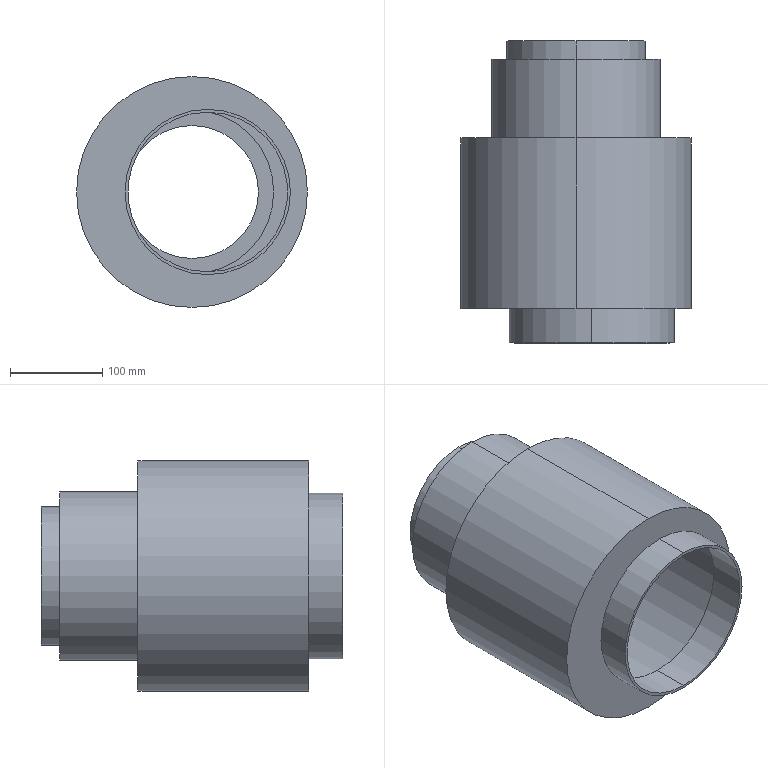Part | SolidWorks | features ICE 1, Revolution 1, Shell 1 | 1 solid | 24 faces | box 250 x 327 x 250 mm | volume 825128 mm3 | cylinder 16 | plane 8 | commonest cylinder face diameters 144 x2 150 x2 173 x2 177 x2 179 x2 183 x2
STEP:
#1=CARTESIAN_POINT('',(17.,-37.,86.5));
#2=VERTEX_POINT('',#1);
#3=CARTESIAN_POINT('',(17.,-37.,-86.5));
#4=VERTEX_POINT('',#3);
#5=CARTESIAN_POINT('',(17.,-37.,0.));
#6=DIRECTION('',(0.,-1.,0.));
#7=DIRECTION('',(0.,0.,-1.));
#8=AXIS2_PLACEMENT_3D('',#5,#6,#7);
#9=CIRCLE('',#8,86.5);
#10=EDGE_CURVE('',#2,#4,#9,.T.);
#11=ORIENTED_EDGE('',*,*,#10,.T.);
#12=CARTESIAN_POINT('',(17.,3.,-86.5));
#13=VERTEX_POINT('',#12);
#14=CARTESIAN_POINT('',(17.,-37.,-86.5));
#15=DIRECTION('',(0.,1.,0.));
#16=VECTOR('',#15,1000.);
#17=LINE('',#14,#16);
#18=EDGE_CURVE('',#4,#13,#17,.T.);
#19=ORIENTED_EDGE('',*,*,#18,.T.);
#20=CARTESIAN_POINT('',(17.,3.,86.5));
#21=VERTEX_POINT('',#20);
#22=CARTESIAN_POINT('',(17.,3.,0.));
#23=DIRECTION('',(0.,-1.,0.));
#24=DIRECTION('',(0.,0.,1.));
#25=AXIS2_PLACEMENT_3D('',#22,#23,#24);
#26=CIRCLE('',#25,86.5);
#27=EDGE_CURVE('',#21,#13,#26,.T.);
#28=ORIENTED_EDGE('',*,*,#27,.F.);
#29=CARTESIAN_POINT('',(17.,-37.,86.5));
#30=DIRECTION('',(0.,1.,0.));
#31=VECTOR('',#30,1000.);
#32=LINE('',#29,#31);
#33=EDGE_CURVE('',#2,#21,#32,.T.);
#34=ORIENTED_EDGE('',*,*,#33,.F.);
#35=EDGE_LOOP('',(#11,#19,#28,#34));
#36=FACE_OUTER_BOUND('',#35,.T.);
#37=CARTESIAN_POINT('',(17.,-37.,0.));
#38=DIRECTION('',(0.,1.,0.));
#39=DIRECTION('',(0.,0.,1.));
#40=AXIS2_PLACEMENT_3D('',#37,#38,#39);
#41=CYLINDRICAL_SURFACE('',#40,86.5);
#42=ADVANCED_FACE('',(#36),#41,.F.);
#43=CARTESIAN_POINT('',(0.,267.,-72.));
#44=VERTEX_POINT('',#43);
#45=CARTESIAN_POINT('',(0.,267.,72.));
#46=VERTEX_POINT('',#45);
#47=CARTESIAN_POINT('',(0.,267.,0.));
#48=DIRECTION('',(0.,1.,0.));
#49=DIRECTION('',(0.,0.,-1.));
#50=AXIS2_PLACEMENT_3D('',#47,#48,#49);
#51=CIRCLE('',#50,72.);
#52=EDGE_CURVE('',#44,#46,#51,.T.);
#53=ORIENTED_EDGE('',*,*,#52,.F.);
#54=CARTESIAN_POINT('',(0.,290.,-72.));
#55=VERTEX_POINT('',#54);
#56=CARTESIAN_POINT('',(0.,290.,-72.));
#57=DIRECTION('',(0.,1.,0.));
#58=VECTOR('',#57,1000.);
#59=LINE('',#56,#58);
#60=EDGE_CURVE('',#44,#55,#59,.T.);
#61=ORIENTED_EDGE('',*,*,#60,.T.);
#62=CARTESIAN_POINT('',(0.,290.,72.));
#63=VERTEX_POINT('',#62);
#64=CARTESIAN_POINT('',(0.,290.,0.));
#65=DIRECTION('',(0.,1.,0.));
#66=DIRECTION('',(0.,0.,-1.));
#67=AXIS2_PLACEMENT_3D('',#64,#65,#66);
#68=CIRCLE('',#67,72.);
#69=EDGE_CURVE('',#55,#63,#68,.T.);
#70=ORIENTED_EDGE('',*,*,#69,.T.);
#71=CARTESIAN_POINT('',(0.,290.,72.));
#72=DIRECTION('',(0.,1.,0.));
#73=VECTOR('',#72,1000.);
#74=LINE('',#71,#73);
#75=EDGE_CURVE('',#46,#63,#74,.T.);
#76=ORIENTED_EDGE('',*,*,#75,.F.);
#77=EDGE_LOOP('',(#53,#61,#70,#76));
#78=FACE_OUTER_BOUND('',#77,.T.);
#79=CARTESIAN_POINT('',(0.,290.,0.));
#80=DIRECTION('',(0.,1.,0.));
#81=DIRECTION('',(0.,0.,1.));
#82=AXIS2_PLACEMENT_3D('',#79,#80,#81);
#83=CYLINDRICAL_SURFACE('',#82,72.);
#84=ADVANCED_FACE('',(#78),#83,.F.);
#85=CARTESIAN_POINT('',(0.,182.,-88.5));
#86=VERTEX_POINT('',#85);
#87=CARTESIAN_POINT('',(0.,182.,88.5));
#88=VERTEX_POINT('',#87);
#89=CARTESIAN_POINT('',(0.,182.,0.));
#90=DIRECTION('',(0.,1.,0.));
#91=DIRECTION('',(0.,0.,-1.));
#92=AXIS2_PLACEMENT_3D('',#89,#90,#91);
#93=CIRCLE('',#92,88.5);
#94=EDGE_CURVE('',#86,#88,#93,.T.);
#95=ORIENTED_EDGE('',*,*,#94,.F.);
#96=CARTESIAN_POINT('',(0.,267.,-88.5));
#97=VERTEX_POINT('',#96);
#98=CARTESIAN_POINT('',(0.,290.,-88.5));
#99=DIRECTION('',(0.,1.,0.));
#100=VECTOR('',#99,1000.);
#101=LINE('',#98,#100);
#102=EDGE_CURVE('',#86,#97,#101,.T.);
#103=ORIENTED_EDGE('',*,*,#102,.T.);
#104=CARTESIAN_POINT('',(0.,267.,88.5));
#105=VERTEX_POINT('',#104);
#106=CARTESIAN_POINT('',(0.,267.,0.));
#107=DIRECTION('',(0.,1.,0.));
#108=DIRECTION('',(0.,0.,-1.));
#109=AXIS2_PLACEMENT_3D('',#106,#107,#108);
#110=CIRCLE('',#109,88.5);
#111=EDGE_CURVE('',#97,#105,#110,.T.);
#112=ORIENTED_EDGE('',*,*,#111,.T.);
#113=CARTESIAN_POINT('',(0.,290.,88.5));
#114=DIRECTION('',(0.,1.,0.));
#115=VECTOR('',#114,1000.);
#116=LINE('',#113,#115);
#117=EDGE_CURVE('',#88,#105,#116,.T.);
#118=ORIENTED_EDGE('',*,*,#117,.F.);
#119=EDGE_LOOP('',(#95,#103,#112,#118));
#120=FACE_OUTER_BOUND('',#119,.T.);
#121=CARTESIAN_POINT('',(0.,290.,0.));
#122=DIRECTION('',(0.,1.,0.));
#123=DIRECTION('',(0.,0.,1.));
#124=AXIS2_PLACEMENT_3D('',#121,#122,#123);
#125=CYLINDRICAL_SURFACE('',#124,88.5);
#126=ADVANCED_FACE('',(#120),#125,.F.);
#127=CARTESIAN_POINT('',(0.,3.,-122.));
#128=VERTEX_POINT('',#127);
#129=CARTESIAN_POINT('',(0.,3.,122.));
#130=VERTEX_POINT('',#129);
#131=CARTESIAN_POINT('',(0.,3.,0.));
#132=DIRECTION('',(0.,1.,0.));
#133=DIRECTION('',(0.,0.,1.));
#134=AXIS2_PLACEMENT_3D('',#131,#132,#133);
#135=CIRCLE('',#134,122.);
#136=EDGE_CURVE('',#128,#130,#135,.T.);
#137=ORIENTED_EDGE('',*,*,#136,.F.);
#138=CARTESIAN_POINT('',(0.,182.,-122.));
#139=VERTEX_POINT('',#138);
#140=CARTESIAN_POINT('',(0.,290.,-122.));
#141=DIRECTION('',(0.,1.,0.));
#142=VECTOR('',#141,1000.);
#143=LINE('',#140,#142);
#144=EDGE_CURVE('',#128,#139,#143,.T.);
#145=ORIENTED_EDGE('',*,*,#144,.T.);
#146=CARTESIAN_POINT('',(0.,182.,122.));
#147=VERTEX_POINT('',#146);
#148=CARTESIAN_POINT('',(0.,182.,0.));
#149=DIRECTION('',(0.,1.,0.));
#150=DIRECTION('',(0.,0.,-1.));
#151=AXIS2_PLACEMENT_3D('',#148,#149,#150);
#152=CIRCLE('',#151,122.);
#153=EDGE_CURVE('',#139,#147,#152,.T.);
#154=ORIENTED_EDGE('',*,*,#153,.T.);
#155=CARTESIAN_POINT('',(0.,290.,122.));
#156=DIRECTION('',(0.,1.,0.));
#157=VECTOR('',#156,1000.);
#158=LINE('',#155,#157);
#159=EDGE_CURVE('',#130,#147,#158,.T.);
#160=ORIENTED_EDGE('',*,*,#159,.F.);
#161=EDGE_LOOP('',(#137,#145,#154,#160));
#162=FACE_OUTER_BOUND('',#161,.T.);
#163=CARTESIAN_POINT('',(0.,290.,0.));
#164=DIRECTION('',(0.,1.,0.));
#165=DIRECTION('',(0.,0.,1.));
#166=AXIS2_PLACEMENT_3D('',#163,#164,#165);
#167=CYLINDRICAL_SURFACE('',#166,122.);
#168=ADVANCED_FACE('',(#162),#167,.F.);
#169=CARTESIAN_POINT('',(17.,-37.,-89.5));
#170=VERTEX_POINT('',#169);
#171=CARTESIAN_POINT('',(17.,-37.,89.5));
#172=VERTEX_POINT('',#171);
#173=CARTESIAN_POINT('',(17.,-37.,0.));
#174=DIRECTION('',(0.,-1.,0.));
#175=DIRECTION('',(0.,0.,-1.));
#176=AXIS2_PLACEMENT_3D('',#173,#174,#175);
#177=CIRCLE('',#176,89.5);
#178=EDGE_CURVE('',#170,#172,#177,.T.);
#179=ORIENTED_EDGE('',*,*,#178,.F.);
#180=CARTESIAN_POINT('',(17.,0.,-89.5));
#181=VERTEX_POINT('',#180);
#182=CARTESIAN_POINT('',(17.,-37.,-89.5));
#183=DIRECTION('',(0.,1.,0.));
#184=VECTOR('',#183,1000.);
#185=LINE('',#182,#184);
#186=EDGE_CURVE('',#170,#181,#185,.T.);
#187=ORIENTED_EDGE('',*,*,#186,.T.);
#188=CARTESIAN_POINT('',(17.,0.,89.5));
#189=VERTEX_POINT('',#188);
#190=CARTESIAN_POINT('',(17.,0.,0.));
#191=DIRECTION('',(0.,-1.,0.));
#192=DIRECTION('',(0.,0.,1.));
#193=AXIS2_PLACEMENT_3D('',#190,#191,#192);
#194=CIRCLE('',#193,89.5);
#195=EDGE_CURVE('',#181,#189,#194,.T.);
#196=ORIENTED_EDGE('',*,*,#195,.T.);
#197=CARTESIAN_POINT('',(17.,-37.,89.5));
#198=DIRECTION('',(0.,1.,0.));
#199=VECTOR('',#198,1000.);
#200=LINE('',#197,#199);
#201=EDGE_CURVE('',#172,#189,#200,.T.);
#202=ORIENTED_EDGE('',*,*,#201,.F.);
#203=EDGE_LOOP('',(#179,#187,#196,#202));
#204=FACE_OUTER_BOUND('',#203,.T.);
#205=CARTESIAN_POINT('',(17.,-37.,0.));
#206=DIRECTION('',(0.,1.,0.));
#207=DIRECTION('',(0.,0.,1.));
#208=AXIS2_PLACEMENT_3D('',#205,#206,#207);
#209=CYLINDRICAL_SURFACE('',#208,89.5);
#210=ADVANCED_FACE('',(#204),#209,.T.);
#211=CARTESIAN_POINT('',(0.,270.,75.));
#212=VERTEX_POINT('',#211);
#213=CARTESIAN_POINT('',(0.,270.,-75.));
#214=VERTEX_POINT('',#213);
#215=CARTESIAN_POINT('',(0.,270.,0.));
#216=DIRECTION('',(0.,1.,0.));
#217=DIRECTION('',(0.,0.,1.));
#218=AXIS2_PLACEMENT_3D('',#215,#216,#217);
#219=CIRCLE('',#218,75.);
#220=EDGE_CURVE('',#212,#214,#219,.T.);
#221=ORIENTED_EDGE('',*,*,#220,.T.);
#222=CARTESIAN_POINT('',(0.,290.,-75.));
#223=VERTEX_POINT('',#222);
#224=CARTESIAN_POINT('',(0.,290.,-75.));
#225=DIRECTION('',(0.,1.,0.));
#226=VECTOR('',#225,1000.);
#227=LINE('',#224,#226);
#228=EDGE_CURVE('',#214,#223,#227,.T.);
#229=ORIENTED_EDGE('',*,*,#228,.T.);
#230=CARTESIAN_POINT('',(0.,290.,75.));
#231=VERTEX_POINT('',#230);
#232=CARTESIAN_POINT('',(0.,290.,0.));
#233=DIRECTION('',(0.,1.,0.));
#234=DIRECTION('',(0.,0.,1.));
#235=AXIS2_PLACEMENT_3D('',#232,#233,#234);
#236=CIRCLE('',#235,75.);
#237=EDGE_CURVE('',#231,#223,#236,.T.);
#238=ORIENTED_EDGE('',*,*,#237,.F.);
#239=CARTESIAN_POINT('',(0.,290.,75.));
#240=DIRECTION('',(0.,1.,0.));
#241=VECTOR('',#240,1000.);
#242=LINE('',#239,#241);
#243=EDGE_CURVE('',#212,#231,#242,.T.);
#244=ORIENTED_EDGE('',*,*,#243,.F.);
#245=EDGE_LOOP('',(#221,#229,#238,#244));
#246=FACE_OUTER_BOUND('',#245,.T.);
#247=CARTESIAN_POINT('',(0.,290.,0.));
#248=DIRECTION('',(0.,1.,0.));
#249=DIRECTION('',(0.,0.,1.));
#250=AXIS2_PLACEMENT_3D('',#247,#248,#249);
#251=CYLINDRICAL_SURFACE('',#250,75.);
#252=ADVANCED_FACE('',(#246),#251,.T.);
#253=CARTESIAN_POINT('',(0.,185.,91.5));
#254=VERTEX_POINT('',#253);
#255=CARTESIAN_POINT('',(0.,185.,-91.5));
#256=VERTEX_POINT('',#255);
#257=CARTESIAN_POINT('',(0.,185.,0.));
#258=DIRECTION('',(0.,1.,0.));
#259=DIRECTION('',(0.,0.,1.));
#260=AXIS2_PLACEMENT_3D('',#257,#258,#259);
#261=CIRCLE('',#260,91.5);
#262=EDGE_CURVE('',#254,#256,#261,.T.);
#263=ORIENTED_EDGE('',*,*,#262,.T.);
#264=CARTESIAN_POINT('',(0.,270.,-91.5));
#265=VERTEX_POINT('',#264);
#266=CARTESIAN_POINT('',(0.,290.,-91.5));
#267=DIRECTION('',(0.,1.,0.));
#268=VECTOR('',#267,1000.);
#269=LINE('',#266,#268);
#270=EDGE_CURVE('',#256,#265,#269,.T.);
#271=ORIENTED_EDGE('',*,*,#270,.T.);
#272=CARTESIAN_POINT('',(0.,270.,91.5));
#273=VERTEX_POINT('',#272);
#274=CARTESIAN_POINT('',(0.,270.,0.));
#275=DIRECTION('',(0.,1.,0.));
#276=DIRECTION('',(0.,0.,1.));
#277=AXIS2_PLACEMENT_3D('',#274,#275,#276);
#278=CIRCLE('',#277,91.5);
#279=EDGE_CURVE('',#273,#265,#278,.T.);
#280=ORIENTED_EDGE('',*,*,#279,.F.);
#281=CARTESIAN_POINT('',(0.,290.,91.5));
#282=DIRECTION('',(0.,1.,0.));
#283=VECTOR('',#282,1000.);
#284=LINE('',#281,#283);
#285=EDGE_CURVE('',#254,#273,#284,.T.);
#286=ORIENTED_EDGE('',*,*,#285,.F.);
#287=EDGE_LOOP('',(#263,#271,#280,#286));
#288=FACE_OUTER_BOUND('',#287,.T.);
#289=CARTESIAN_POINT('',(0.,290.,0.));
#290=DIRECTION('',(0.,1.,0.));
#291=DIRECTION('',(0.,0.,1.));
#292=AXIS2_PLACEMENT_3D('',#289,#290,#291);
#293=CYLINDRICAL_SURFACE('',#292,91.5);
#294=ADVANCED_FACE('',(#288),#293,.T.);
#295=CARTESIAN_POINT('',(0.,0.,125.));
#296=VERTEX_POINT('',#295);
#297=CARTESIAN_POINT('',(0.,0.,-125.));
#298=VERTEX_POINT('',#297);
#299=CARTESIAN_POINT('',(0.,0.,0.));
#300=DIRECTION('',(0.,1.,0.));
#301=DIRECTION('',(0.,0.,1.));
#302=AXIS2_PLACEMENT_3D('',#299,#300,#301);
#303=CIRCLE('',#302,125.);
#304=EDGE_CURVE('',#296,#298,#303,.T.);
#305=ORIENTED_EDGE('',*,*,#304,.T.);
#306=CARTESIAN_POINT('',(0.,185.,-125.));
#307=VERTEX_POINT('',#306);
#308=CARTESIAN_POINT('',(0.,290.,-125.));
#309=DIRECTION('',(0.,1.,0.));
#310=VECTOR('',#309,1000.);
#311=LINE('',#308,#310);
#312=EDGE_CURVE('',#298,#307,#311,.T.);
#313=ORIENTED_EDGE('',*,*,#312,.T.);
#314=CARTESIAN_POINT('',(0.,185.,125.));
#315=VERTEX_POINT('',#314);
#316=CARTESIAN_POINT('',(0.,185.,0.));
#317=DIRECTION('',(0.,1.,0.));
#318=DIRECTION('',(0.,0.,1.));
#319=AXIS2_PLACEMENT_3D('',#316,#317,#318);
#320=CIRCLE('',#319,125.);
#321=EDGE_CURVE('',#315,#307,#320,.T.);
#322=ORIENTED_EDGE('',*,*,#321,.F.);
#323=CARTESIAN_POINT('',(0.,290.,125.));
#324=DIRECTION('',(0.,1.,0.));
#325=VECTOR('',#324,1000.);
#326=LINE('',#323,#325);
#327=EDGE_CURVE('',#296,#315,#326,.T.);
#328=ORIENTED_EDGE('',*,*,#327,.F.);
#329=EDGE_LOOP('',(#305,#313,#322,#328));
#330=FACE_OUTER_BOUND('',#329,.T.);
#331=CARTESIAN_POINT('',(0.,290.,0.));
#332=DIRECTION('',(0.,1.,0.));
#333=DIRECTION('',(0.,0.,1.));
#334=AXIS2_PLACEMENT_3D('',#331,#332,#333);
#335=CYLINDRICAL_SURFACE('',#334,125.);
#336=ADVANCED_FACE('',(#330),#335,.T.);
#337=CARTESIAN_POINT('',(17.,0.,0.));
#338=DIRECTION('',(0.,-1.,0.));
#339=DIRECTION('',(0.,0.,1.));
#340=AXIS2_PLACEMENT_3D('',#337,#338,#339);
#341=CIRCLE('',#340,89.5);
#342=EDGE_CURVE('',#189,#181,#341,.T.);
#343=ORIENTED_EDGE('',*,*,#342,.F.);
#344=ORIENTED_EDGE('',*,*,#195,.F.);
#345=EDGE_LOOP('',(#343,#344));
#346=FACE_BOUND('',#345,.T.);
#347=ORIENTED_EDGE('',*,*,#304,.F.);
#348=CARTESIAN_POINT('',(0.,0.,0.));
#349=DIRECTION('',(0.,1.,0.));
#350=DIRECTION('',(0.,0.,1.));
#351=AXIS2_PLACEMENT_3D('',#348,#349,#350);
#352=CIRCLE('',#351,125.);
#353=EDGE_CURVE('',#298,#296,#352,.T.);
#354=ORIENTED_EDGE('',*,*,#353,.F.);
#355=EDGE_LOOP('',(#347,#354));
#356=FACE_OUTER_BOUND('',#355,.T.);
#357=CARTESIAN_POINT('',(0.,0.,0.));
#358=DIRECTION('',(0.,1.,0.));
#359=DIRECTION('',(0.,0.,1.));
#360=AXIS2_PLACEMENT_3D('',#357,#358,#359);
#361=PLANE('',#360);
#362=ADVANCED_FACE('',(#346,#356),#361,.F.);
#363=ORIENTED_EDGE('',*,*,#312,.F.);
#364=ORIENTED_EDGE('',*,*,#353,.T.);
#365=ORIENTED_EDGE('',*,*,#327,.T.);
#366=CARTESIAN_POINT('',(0.,185.,0.));
#367=DIRECTION('',(0.,1.,0.));
#368=DIRECTION('',(0.,0.,1.));
#369=AXIS2_PLACEMENT_3D('',#366,#367,#368);
#370=CIRCLE('',#369,125.);
#371=EDGE_CURVE('',#307,#315,#370,.T.);
#372=ORIENTED_EDGE('',*,*,#371,.F.);
#373=EDGE_LOOP('',(#363,#364,#365,#372));
#374=FACE_OUTER_BOUND('',#373,.T.);
#375=CARTESIAN_POINT('',(0.,290.,0.));
#376=DIRECTION('',(0.,1.,0.));
#377=DIRECTION('',(0.,0.,1.));
#378=AXIS2_PLACEMENT_3D('',#375,#376,#377);
#379=CYLINDRICAL_SURFACE('',#378,125.);
#380=ADVANCED_FACE('',(#374),#379,.T.);
#381=ORIENTED_EDGE('',*,*,#262,.F.);
#382=CARTESIAN_POINT('',(0.,185.,0.));
#383=DIRECTION('',(0.,1.,0.));
#384=DIRECTION('',(0.,0.,1.));
#385=AXIS2_PLACEMENT_3D('',#382,#383,#384);
#386=CIRCLE('',#385,91.5);
#387=EDGE_CURVE('',#256,#254,#386,.T.);
#388=ORIENTED_EDGE('',*,*,#387,.F.);
#389=EDGE_LOOP('',(#381,#388));
#390=FACE_BOUND('',#389,.T.);
#391=ORIENTED_EDGE('',*,*,#321,.T.);
#392=ORIENTED_EDGE('',*,*,#371,.T.);
#393=EDGE_LOOP('',(#391,#392));
#394=FACE_OUTER_BOUND('',#393,.T.);
#395=CARTESIAN_POINT('',(125.,185.,0.));
#396=DIRECTION('',(0.,-1.,0.));
#397=DIRECTION('',(0.,0.,-1.));
#398=AXIS2_PLACEMENT_3D('',#395,#396,#397);
#399=PLANE('',#398);
#400=ADVANCED_FACE('',(#390,#394),#399,.F.);
#401=ORIENTED_EDGE('',*,*,#270,.F.);
#402=ORIENTED_EDGE('',*,*,#387,.T.);
#403=ORIENTED_EDGE('',*,*,#285,.T.);
#404=CARTESIAN_POINT('',(0.,270.,0.));
#405=DIRECTION('',(0.,1.,0.));
#406=DIRECTION('',(0.,0.,1.));
#407=AXIS2_PLACEMENT_3D('',#404,#405,#406);
#408=CIRCLE('',#407,91.5);
#409=EDGE_CURVE('',#265,#273,#408,.T.);
#410=ORIENTED_EDGE('',*,*,#409,.F.);
#411=EDGE_LOOP('',(#401,#402,#403,#410));
#412=FACE_OUTER_BOUND('',#411,.T.);
#413=CARTESIAN_POINT('',(0.,290.,0.));
#414=DIRECTION('',(0.,1.,0.));
#415=DIRECTION('',(0.,0.,1.));
#416=AXIS2_PLACEMENT_3D('',#413,#414,#415);
#417=CYLINDRICAL_SURFACE('',#416,91.5);
#418=ADVANCED_FACE('',(#412),#417,.T.);
#419=ORIENTED_EDGE('',*,*,#220,.F.);
#420=CARTESIAN_POINT('',(0.,270.,0.));
#421=DIRECTION('',(0.,1.,0.));
#422=DIRECTION('',(0.,0.,1.));
#423=AXIS2_PLACEMENT_3D('',#420,#421,#422);
#424=CIRCLE('',#423,75.);
#425=EDGE_CURVE('',#214,#212,#424,.T.);
#426=ORIENTED_EDGE('',*,*,#425,.F.);
#427=EDGE_LOOP('',(#419,#426));
#428=FACE_BOUND('',#427,.T.);
#429=ORIENTED_EDGE('',*,*,#279,.T.);
#430=ORIENTED_EDGE('',*,*,#409,.T.);
#431=EDGE_LOOP('',(#429,#430));
#432=FACE_OUTER_BOUND('',#431,.T.);
#433=CARTESIAN_POINT('',(91.5,270.,0.));
#434=DIRECTION('',(0.,-1.,0.));
#435=DIRECTION('',(0.,0.,-1.));
#436=AXIS2_PLACEMENT_3D('',#433,#434,#435);
#437=PLANE('',#436);
#438=ADVANCED_FACE('',(#428,#432),#437,.F.);
#439=ORIENTED_EDGE('',*,*,#228,.F.);
#440=ORIENTED_EDGE('',*,*,#425,.T.);
#441=ORIENTED_EDGE('',*,*,#243,.T.);
#442=CARTESIAN_POINT('',(0.,290.,0.));
#443=DIRECTION('',(0.,1.,0.));
#444=DIRECTION('',(0.,0.,1.));
#445=AXIS2_PLACEMENT_3D('',#442,#443,#444);
#446=CIRCLE('',#445,75.);
#447=EDGE_CURVE('',#223,#231,#446,.T.);
#448=ORIENTED_EDGE('',*,*,#447,.F.);
#449=EDGE_LOOP('',(#439,#440,#441,#448));
#450=FACE_OUTER_BOUND('',#449,.T.);
#451=CARTESIAN_POINT('',(0.,290.,0.));
#452=DIRECTION('',(0.,1.,0.));
#453=DIRECTION('',(0.,0.,1.));
#454=AXIS2_PLACEMENT_3D('',#451,#452,#453);
#455=CYLINDRICAL_SURFACE('',#454,75.);
#456=ADVANCED_FACE('',(#450),#455,.T.);
#457=CARTESIAN_POINT('',(0.,290.,0.));
#458=DIRECTION('',(0.,1.,0.));
#459=DIRECTION('',(0.,0.,-1.));
#460=AXIS2_PLACEMENT_3D('',#457,#458,#459);
#461=CIRCLE('',#460,72.);
#462=EDGE_CURVE('',#63,#55,#461,.T.);
#463=ORIENTED_EDGE('',*,*,#462,.F.);
#464=ORIENTED_EDGE('',*,*,#69,.F.);
#465=EDGE_LOOP('',(#463,#464));
#466=FACE_BOUND('',#465,.T.);
#467=ORIENTED_EDGE('',*,*,#237,.T.);
#468=ORIENTED_EDGE('',*,*,#447,.T.);
#469=EDGE_LOOP('',(#467,#468));
#470=FACE_OUTER_BOUND('',#469,.T.);
#471=CARTESIAN_POINT('',(75.,290.,0.));
#472=DIRECTION('',(0.,-1.,0.));
#473=DIRECTION('',(0.,0.,-1.));
#474=AXIS2_PLACEMENT_3D('',#471,#472,#473);
#475=PLANE('',#474);
#476=ADVANCED_FACE('',(#466,#470),#475,.F.);
#477=ORIENTED_EDGE('',*,*,#186,.F.);
#478=CARTESIAN_POINT('',(17.,-37.,0.));
#479=DIRECTION('',(0.,-1.,0.));
#480=DIRECTION('',(0.,0.,-1.));
#481=AXIS2_PLACEMENT_3D('',#478,#479,#480);
#482=CIRCLE('',#481,89.5);
#483=EDGE_CURVE('',#172,#170,#482,.T.);
#484=ORIENTED_EDGE('',*,*,#483,.F.);
#485=ORIENTED_EDGE('',*,*,#201,.T.);
#486=ORIENTED_EDGE('',*,*,#342,.T.);
#487=EDGE_LOOP('',(#477,#484,#485,#486));
#488=FACE_OUTER_BOUND('',#487,.T.);
#489=CARTESIAN_POINT('',(17.,-37.,0.));
#490=DIRECTION('',(0.,1.,0.));
#491=DIRECTION('',(0.,0.,1.));
#492=AXIS2_PLACEMENT_3D('',#489,#490,#491);
#493=CYLINDRICAL_SURFACE('',#492,89.5);
#494=ADVANCED_FACE('',(#488),#493,.T.);
#495=ORIENTED_EDGE('',*,*,#10,.F.);
#496=CARTESIAN_POINT('',(17.,-37.,0.));
#497=DIRECTION('',(0.,-1.,0.));
#498=DIRECTION('',(0.,0.,-1.));
#499=AXIS2_PLACEMENT_3D('',#496,#497,#498);
#500=CIRCLE('',#499,86.5);
#501=EDGE_CURVE('',#4,#2,#500,.T.);
#502=ORIENTED_EDGE('',*,*,#501,.F.);
#503=EDGE_LOOP('',(#495,#502));
#504=FACE_BOUND('',#503,.T.);
#505=ORIENTED_EDGE('',*,*,#483,.T.);
#506=ORIENTED_EDGE('',*,*,#178,.T.);
#507=EDGE_LOOP('',(#505,#506));
#508=FACE_OUTER_BOUND('',#507,.T.);
#509=CARTESIAN_POINT('',(17.,-37.,0.));
#510=DIRECTION('',(0.,-1.,0.));
#511=DIRECTION('',(0.,0.,-1.));
#512=AXIS2_PLACEMENT_3D('',#509,#510,#511);
#513=PLANE('',#512);
#514=ADVANCED_FACE('',(#504,#508),#513,.T.);
#515=ORIENTED_EDGE('',*,*,#27,.T.);
#516=CARTESIAN_POINT('',(17.,3.,0.));
#517=DIRECTION('',(0.,-1.,0.));
#518=DIRECTION('',(0.,0.,1.));
#519=AXIS2_PLACEMENT_3D('',#516,#517,#518);
#520=CIRCLE('',#519,86.5);
#521=EDGE_CURVE('',#13,#21,#520,.T.);
#522=ORIENTED_EDGE('',*,*,#521,.T.);
#523=EDGE_LOOP('',(#515,#522));
#524=FACE_BOUND('',#523,.T.);
#525=CARTESIAN_POINT('',(0.,3.,0.));
#526=DIRECTION('',(0.,1.,0.));
#527=DIRECTION('',(0.,0.,1.));
#528=AXIS2_PLACEMENT_3D('',#525,#526,#527);
#529=CIRCLE('',#528,122.);
#530=EDGE_CURVE('',#130,#128,#529,.T.);
#531=ORIENTED_EDGE('',*,*,#530,.T.);
#532=ORIENTED_EDGE('',*,*,#136,.T.);
#533=EDGE_LOOP('',(#531,#532));
#534=FACE_OUTER_BOUND('',#533,.T.);
#535=CARTESIAN_POINT('',(0.,3.,0.));
#536=DIRECTION('',(0.,1.,0.));
#537=DIRECTION('',(0.,0.,1.));
#538=AXIS2_PLACEMENT_3D('',#535,#536,#537);
#539=PLANE('',#538);
#540=ADVANCED_FACE('',(#524,#534),#539,.T.);
#541=ORIENTED_EDGE('',*,*,#144,.F.);
#542=ORIENTED_EDGE('',*,*,#530,.F.);
#543=ORIENTED_EDGE('',*,*,#159,.T.);
#544=CARTESIAN_POINT('',(0.,182.,0.));
#545=DIRECTION('',(0.,1.,0.));
#546=DIRECTION('',(0.,0.,-1.));
#547=AXIS2_PLACEMENT_3D('',#544,#545,#546);
#548=CIRCLE('',#547,122.);
#549=EDGE_CURVE('',#147,#139,#548,.T.);
#550=ORIENTED_EDGE('',*,*,#549,.T.);
#551=EDGE_LOOP('',(#541,#542,#543,#550));
#552=FACE_OUTER_BOUND('',#551,.T.);
#553=CARTESIAN_POINT('',(0.,290.,0.));
#554=DIRECTION('',(0.,1.,0.));
#555=DIRECTION('',(0.,0.,1.));
#556=AXIS2_PLACEMENT_3D('',#553,#554,#555);
#557=CYLINDRICAL_SURFACE('',#556,122.);
#558=ADVANCED_FACE('',(#552),#557,.F.);
#559=CARTESIAN_POINT('',(0.,182.,0.));
#560=DIRECTION('',(0.,1.,0.));
#561=DIRECTION('',(0.,0.,-1.));
#562=AXIS2_PLACEMENT_3D('',#559,#560,#561);
#563=CIRCLE('',#562,88.5);
#564=EDGE_CURVE('',#88,#86,#563,.T.);
#565=ORIENTED_EDGE('',*,*,#564,.T.);
#566=ORIENTED_EDGE('',*,*,#94,.T.);
#567=EDGE_LOOP('',(#565,#566));
#568=FACE_BOUND('',#567,.T.);
#569=ORIENTED_EDGE('',*,*,#549,.F.);
#570=ORIENTED_EDGE('',*,*,#153,.F.);
#571=EDGE_LOOP('',(#569,#570));
#572=FACE_OUTER_BOUND('',#571,.T.);
#573=CARTESIAN_POINT('',(125.,182.,0.));
#574=DIRECTION('',(0.,-1.,0.));
#575=DIRECTION('',(0.,0.,-1.));
#576=AXIS2_PLACEMENT_3D('',#573,#574,#575);
#577=PLANE('',#576);
#578=ADVANCED_FACE('',(#568,#572),#577,.T.);
#579=ORIENTED_EDGE('',*,*,#102,.F.);
#580=ORIENTED_EDGE('',*,*,#564,.F.);
#581=ORIENTED_EDGE('',*,*,#117,.T.);
#582=CARTESIAN_POINT('',(0.,267.,0.));
#583=DIRECTION('',(0.,1.,0.));
#584=DIRECTION('',(0.,0.,-1.));
#585=AXIS2_PLACEMENT_3D('',#582,#583,#584);
#586=CIRCLE('',#585,88.5);
#587=EDGE_CURVE('',#105,#97,#586,.T.);
#588=ORIENTED_EDGE('',*,*,#587,.T.);
#589=EDGE_LOOP('',(#579,#580,#581,#588));
#590=FACE_OUTER_BOUND('',#589,.T.);
#591=CARTESIAN_POINT('',(0.,290.,0.));
#592=DIRECTION('',(0.,1.,0.));
#593=DIRECTION('',(0.,0.,1.));
#594=AXIS2_PLACEMENT_3D('',#591,#592,#593);
#595=CYLINDRICAL_SURFACE('',#594,88.5);
#596=ADVANCED_FACE('',(#590),#595,.F.);
#597=CARTESIAN_POINT('',(0.,267.,0.));
#598=DIRECTION('',(0.,1.,0.));
#599=DIRECTION('',(0.,0.,-1.));
#600=AXIS2_PLACEMENT_3D('',#597,#598,#599);
#601=CIRCLE('',#600,72.);
#602=EDGE_CURVE('',#46,#44,#601,.T.);
#603=ORIENTED_EDGE('',*,*,#602,.T.);
#604=ORIENTED_EDGE('',*,*,#52,.T.);
#605=EDGE_LOOP('',(#603,#604));
#606=FACE_BOUND('',#605,.T.);
#607=ORIENTED_EDGE('',*,*,#587,.F.);
#608=ORIENTED_EDGE('',*,*,#111,.F.);
#609=EDGE_LOOP('',(#607,#608));
#610=FACE_OUTER_BOUND('',#609,.T.);
#611=CARTESIAN_POINT('',(91.5,267.,0.));
#612=DIRECTION('',(0.,-1.,0.));
#613=DIRECTION('',(0.,0.,-1.));
#614=AXIS2_PLACEMENT_3D('',#611,#612,#613);
#615=PLANE('',#614);
#616=ADVANCED_FACE('',(#606,#610),#615,.T.);
#617=ORIENTED_EDGE('',*,*,#60,.F.);
#618=ORIENTED_EDGE('',*,*,#602,.F.);
#619=ORIENTED_EDGE('',*,*,#75,.T.);
#620=ORIENTED_EDGE('',*,*,#462,.T.);
#621=EDGE_LOOP('',(#617,#618,#619,#620));
#622=FACE_OUTER_BOUND('',#621,.T.);
#623=CARTESIAN_POINT('',(0.,290.,0.));
#624=DIRECTION('',(0.,1.,0.));
#625=DIRECTION('',(0.,0.,1.));
#626=AXIS2_PLACEMENT_3D('',#623,#624,#625);
#627=CYLINDRICAL_SURFACE('',#626,72.);
#628=ADVANCED_FACE('',(#622),#627,.F.);
#629=ORIENTED_EDGE('',*,*,#18,.F.);
#630=ORIENTED_EDGE('',*,*,#501,.T.);
#631=ORIENTED_EDGE('',*,*,#33,.T.);
#632=ORIENTED_EDGE('',*,*,#521,.F.);
#633=EDGE_LOOP('',(#629,#630,#631,#632));
#634=FACE_OUTER_BOUND('',#633,.T.);
#635=CARTESIAN_POINT('',(17.,-37.,0.));
#636=DIRECTION('',(0.,1.,0.));
#637=DIRECTION('',(0.,0.,1.));
#638=AXIS2_PLACEMENT_3D('',#635,#636,#637);
#639=CYLINDRICAL_SURFACE('',#638,86.5);
#640=ADVANCED_FACE('',(#634),#639,.F.);
#641=CLOSED_SHELL('',(#42,#84,#126,#168,#210,#252,#294,#336,#362,#380,#400,#418,#438,#456,#476,#494,#514,#540,#558,#578,#596,#616,#628,#640));
#642=MANIFOLD_SOLID_BREP('',#641);
#643=CARTESIAN_POINT('',(0.,0.,0.));
#644=DIRECTION('',(0.,0.,1.));
#645=DIRECTION('',(1.,0.,0.));
#646=AXIS2_PLACEMENT_3D('',#643,#644,#645);
#647=(LENGTH_UNIT()NAMED_UNIT(*)SI_UNIT(.MILLI.,.METRE.));
#648=UNCERTAINTY_MEASURE_WITH_UNIT(LENGTH_MEASURE(0.00001),#647,'','');
#649=(NAMED_UNIT(*)PLANE_ANGLE_UNIT()SI_UNIT($,.RADIAN.));
#650=(NAMED_UNIT(*)SI_UNIT($,.STERADIAN.)SOLID_ANGLE_UNIT());
#651=(GEOMETRIC_REPRESENTATION_CONTEXT(3)GLOBAL_UNCERTAINTY_ASSIGNED_CONTEXT((#648))GLOBAL_UNIT_ASSIGNED_CONTEXT((#647,#649,#650))REPRESENTATION_CONTEXT('',''));
#652=ADVANCED_BREP_SHAPE_REPRESENTATION('',(#642,#646),#651);